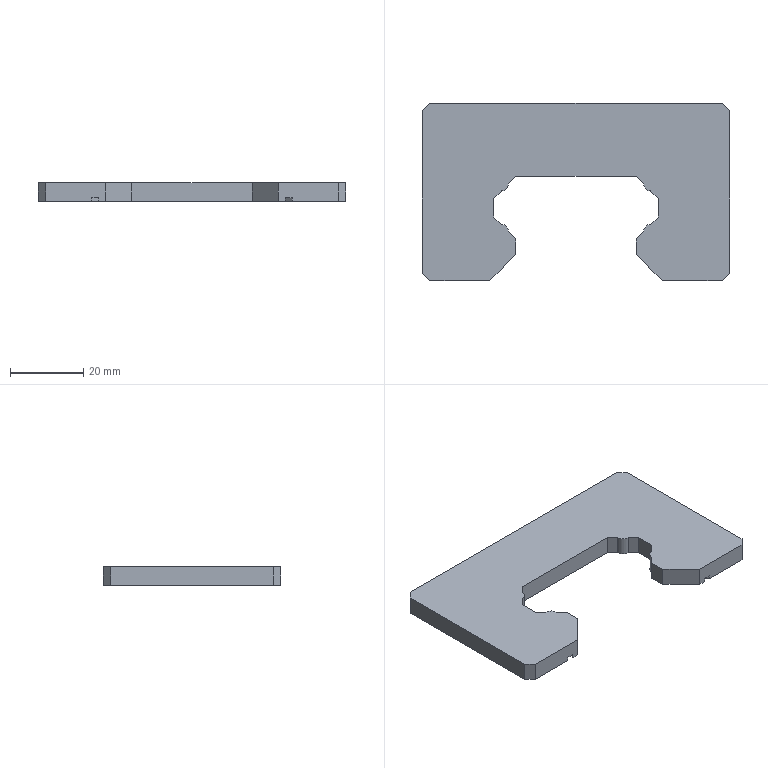Part | SolidWorks | features SplitBody 1 | 1 solid | 104 faces | box 84.105 x 48.48 x 5.05 mm | volume 14009 mm3 | plane 81 | cylinder 15 | torus 4 | sphere 4 | commonest cylinder face diameters 3.924 x6 6.384 x4 7.98 x4 13 x1